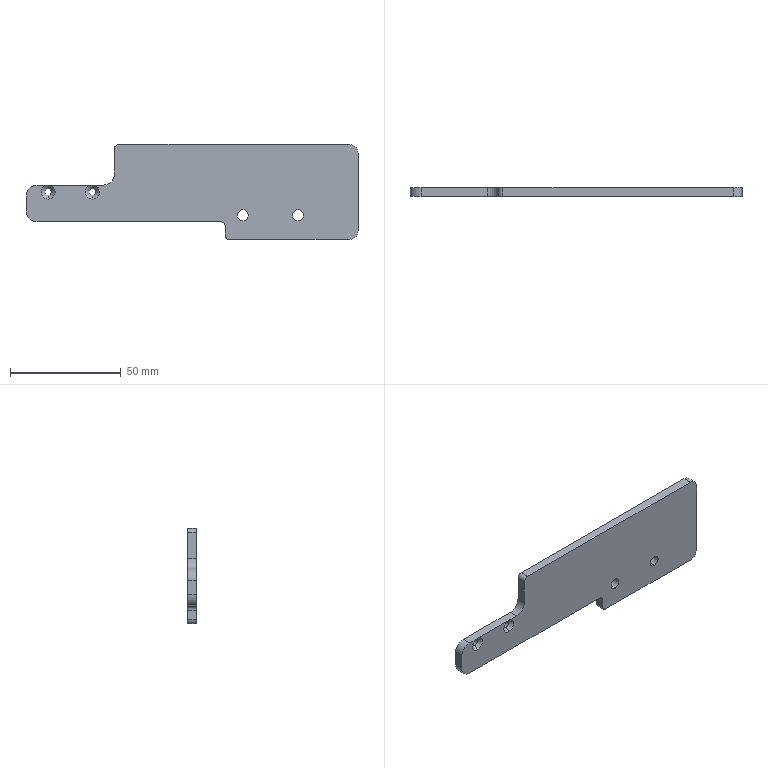Part | SolidWorks | features BaseBody 1 | 1 solid | 30 faces | box 150 x 4 x 43 mm | volume 19674 mm3 | cylinder 16 | plane 10 | cone 4 | commonest cylinder face diameters 3.1 x4 5 x4 4 x3 10 x3 8 x2
STEP:
#1=CARTESIAN_POINT('',(-78.,1.65,-1.55));
#2=VERTEX_POINT('',#1);
#3=CARTESIAN_POINT('',(-78.,1.65,1.55));
#4=VERTEX_POINT('',#3);
#5=CARTESIAN_POINT('',(-78.,1.65,0.));
#6=DIRECTION('',(0.,1.,0.));
#7=DIRECTION('',(0.,0.,1.));
#8=AXIS2_PLACEMENT_3D('',#5,#6,#7);
#9=CIRCLE('',#8,1.55);
#10=EDGE_CURVE('',#2,#4,#9,.T.);
#11=ORIENTED_EDGE('',*,*,#10,.F.);
#12=CARTESIAN_POINT('',(-78.,4.,-1.55));
#13=VERTEX_POINT('',#12);
#14=CARTESIAN_POINT('',(-78.,0.,-1.55));
#15=DIRECTION('',(0.,1.,0.));
#16=VECTOR('',#15,1000.);
#17=LINE('',#14,#16);
#18=EDGE_CURVE('',#2,#13,#17,.T.);
#19=ORIENTED_EDGE('',*,*,#18,.T.);
#20=CARTESIAN_POINT('',(-78.,4.,1.55));
#21=VERTEX_POINT('',#20);
#22=CARTESIAN_POINT('',(-78.,4.,0.));
#23=DIRECTION('',(0.,1.,0.));
#24=DIRECTION('',(0.,0.,1.));
#25=AXIS2_PLACEMENT_3D('',#22,#23,#24);
#26=CIRCLE('',#25,1.55);
#27=EDGE_CURVE('',#13,#21,#26,.T.);
#28=ORIENTED_EDGE('',*,*,#27,.T.);
#29=CARTESIAN_POINT('',(-78.,0.,1.55));
#30=DIRECTION('',(0.,1.,0.));
#31=VECTOR('',#30,1000.);
#32=LINE('',#29,#31);
#33=EDGE_CURVE('',#4,#21,#32,.T.);
#34=ORIENTED_EDGE('',*,*,#33,.F.);
#35=EDGE_LOOP('',(#11,#19,#28,#34));
#36=FACE_OUTER_BOUND('',#35,.T.);
#37=CARTESIAN_POINT('',(-78.,0.,0.));
#38=DIRECTION('',(0.,1.,0.));
#39=DIRECTION('',(0.,0.,1.));
#40=AXIS2_PLACEMENT_3D('',#37,#38,#39);
#41=CYLINDRICAL_SURFACE('',#40,1.55);
#42=ADVANCED_FACE('',(#36),#41,.F.);
#43=CARTESIAN_POINT('',(-98.,1.65,-1.55));
#44=VERTEX_POINT('',#43);
#45=CARTESIAN_POINT('',(-98.,1.65,1.55));
#46=VERTEX_POINT('',#45);
#47=CARTESIAN_POINT('',(-98.,1.65,0.));
#48=DIRECTION('',(0.,1.,0.));
#49=DIRECTION('',(0.,0.,1.));
#50=AXIS2_PLACEMENT_3D('',#47,#48,#49);
#51=CIRCLE('',#50,1.55);
#52=EDGE_CURVE('',#44,#46,#51,.T.);
#53=ORIENTED_EDGE('',*,*,#52,.F.);
#54=CARTESIAN_POINT('',(-98.,4.,-1.55));
#55=VERTEX_POINT('',#54);
#56=CARTESIAN_POINT('',(-98.,0.,-1.55));
#57=DIRECTION('',(0.,1.,0.));
#58=VECTOR('',#57,1000.);
#59=LINE('',#56,#58);
#60=EDGE_CURVE('',#44,#55,#59,.T.);
#61=ORIENTED_EDGE('',*,*,#60,.T.);
#62=CARTESIAN_POINT('',(-98.,4.,1.55));
#63=VERTEX_POINT('',#62);
#64=CARTESIAN_POINT('',(-98.,4.,0.));
#65=DIRECTION('',(0.,1.,0.));
#66=DIRECTION('',(0.,0.,1.));
#67=AXIS2_PLACEMENT_3D('',#64,#65,#66);
#68=CIRCLE('',#67,1.55);
#69=EDGE_CURVE('',#55,#63,#68,.T.);
#70=ORIENTED_EDGE('',*,*,#69,.T.);
#71=CARTESIAN_POINT('',(-98.,0.,1.55));
#72=DIRECTION('',(0.,1.,0.));
#73=VECTOR('',#72,1000.);
#74=LINE('',#71,#73);
#75=EDGE_CURVE('',#46,#63,#74,.T.);
#76=ORIENTED_EDGE('',*,*,#75,.F.);
#77=EDGE_LOOP('',(#53,#61,#70,#76));
#78=FACE_OUTER_BOUND('',#77,.T.);
#79=CARTESIAN_POINT('',(-98.,0.,0.));
#80=DIRECTION('',(0.,1.,0.));
#81=DIRECTION('',(0.,0.,1.));
#82=AXIS2_PLACEMENT_3D('',#79,#80,#81);
#83=CYLINDRICAL_SURFACE('',#82,1.55);
#84=ADVANCED_FACE('',(#78),#83,.F.);
#85=CARTESIAN_POINT('',(14.95,4.,-13.));
#86=VERTEX_POINT('',#85);
#87=CARTESIAN_POINT('',(14.95,4.,-8.));
#88=VERTEX_POINT('',#87);
#89=CARTESIAN_POINT('',(14.95,4.,-10.5));
#90=DIRECTION('',(0.,1.,0.));
#91=DIRECTION('',(0.,0.,-1.));
#92=AXIS2_PLACEMENT_3D('',#89,#90,#91);
#93=CIRCLE('',#92,2.5);
#94=EDGE_CURVE('',#86,#88,#93,.T.);
#95=ORIENTED_EDGE('',*,*,#94,.T.);
#96=CARTESIAN_POINT('',(14.95,0.,-8.));
#97=VERTEX_POINT('',#96);
#98=CARTESIAN_POINT('',(14.95,10.,-8.));
#99=DIRECTION('',(0.,-1.,0.));
#100=VECTOR('',#99,1000.);
#101=LINE('',#98,#100);
#102=EDGE_CURVE('',#88,#97,#101,.T.);
#103=ORIENTED_EDGE('',*,*,#102,.T.);
#104=CARTESIAN_POINT('',(14.95,0.,-13.));
#105=VERTEX_POINT('',#104);
#106=CARTESIAN_POINT('',(14.95,0.,-10.5));
#107=DIRECTION('',(0.,1.,0.));
#108=DIRECTION('',(0.,0.,-1.));
#109=AXIS2_PLACEMENT_3D('',#106,#107,#108);
#110=CIRCLE('',#109,2.5);
#111=EDGE_CURVE('',#105,#97,#110,.T.);
#112=ORIENTED_EDGE('',*,*,#111,.F.);
#113=CARTESIAN_POINT('',(14.95,10.,-13.));
#114=DIRECTION('',(0.,-1.,0.));
#115=VECTOR('',#114,1000.);
#116=LINE('',#113,#115);
#117=EDGE_CURVE('',#86,#105,#116,.T.);
#118=ORIENTED_EDGE('',*,*,#117,.F.);
#119=EDGE_LOOP('',(#95,#103,#112,#118));
#120=FACE_OUTER_BOUND('',#119,.T.);
#121=CARTESIAN_POINT('',(14.95,10.,-10.5));
#122=DIRECTION('',(0.,-1.,0.));
#123=DIRECTION('',(0.,0.,-1.));
#124=AXIS2_PLACEMENT_3D('',#121,#122,#123);
#125=CYLINDRICAL_SURFACE('',#124,2.5);
#126=ADVANCED_FACE('',(#120),#125,.F.);
#127=CARTESIAN_POINT('',(-10.05,4.,-13.));
#128=VERTEX_POINT('',#127);
#129=CARTESIAN_POINT('',(-10.05,4.,-8.));
#130=VERTEX_POINT('',#129);
#131=CARTESIAN_POINT('',(-10.05,4.,-10.5));
#132=DIRECTION('',(0.,1.,0.));
#133=DIRECTION('',(0.,0.,-1.));
#134=AXIS2_PLACEMENT_3D('',#131,#132,#133);
#135=CIRCLE('',#134,2.5);
#136=EDGE_CURVE('',#128,#130,#135,.T.);
#137=ORIENTED_EDGE('',*,*,#136,.T.);
#138=CARTESIAN_POINT('',(-10.05,0.,-8.));
#139=VERTEX_POINT('',#138);
#140=CARTESIAN_POINT('',(-10.05,10.,-8.));
#141=DIRECTION('',(0.,-1.,0.));
#142=VECTOR('',#141,1000.);
#143=LINE('',#140,#142);
#144=EDGE_CURVE('',#130,#139,#143,.T.);
#145=ORIENTED_EDGE('',*,*,#144,.T.);
#146=CARTESIAN_POINT('',(-10.05,0.,-13.));
#147=VERTEX_POINT('',#146);
#148=CARTESIAN_POINT('',(-10.05,0.,-10.5));
#149=DIRECTION('',(0.,1.,0.));
#150=DIRECTION('',(0.,0.,-1.));
#151=AXIS2_PLACEMENT_3D('',#148,#149,#150);
#152=CIRCLE('',#151,2.5);
#153=EDGE_CURVE('',#147,#139,#152,.T.);
#154=ORIENTED_EDGE('',*,*,#153,.F.);
#155=CARTESIAN_POINT('',(-10.05,10.,-13.));
#156=DIRECTION('',(0.,-1.,0.));
#157=VECTOR('',#156,1000.);
#158=LINE('',#155,#157);
#159=EDGE_CURVE('',#128,#147,#158,.T.);
#160=ORIENTED_EDGE('',*,*,#159,.F.);
#161=EDGE_LOOP('',(#137,#145,#154,#160));
#162=FACE_OUTER_BOUND('',#161,.T.);
#163=CARTESIAN_POINT('',(-10.05,10.,-10.5));
#164=DIRECTION('',(0.,-1.,0.));
#165=DIRECTION('',(0.,0.,-1.));
#166=AXIS2_PLACEMENT_3D('',#163,#164,#165);
#167=CYLINDRICAL_SURFACE('',#166,2.5);
#168=ADVANCED_FACE('',(#162),#167,.F.);
#169=ORIENTED_EDGE('',*,*,#10,.T.);
#170=CARTESIAN_POINT('',(-78.,0.07698,3.123));
#171=VERTEX_POINT('',#170);
#172=CARTESIAN_POINT('',(-78.,0.,3.2));
#173=DIRECTION('',(0.,-0.7071,0.7071));
#174=VECTOR('',#173,1000.);
#175=LINE('',#172,#174);
#176=EDGE_CURVE('',#4,#171,#175,.T.);
#177=ORIENTED_EDGE('',*,*,#176,.T.);
#178=CARTESIAN_POINT('',(-78.698,0.,3.123));
#179=VERTEX_POINT('',#178);
#180=CARTESIAN_POINT('',(-78.698,0.,3.123));
#181=CARTESIAN_POINT('',(-78.468,0.05012,3.123));
#182=CARTESIAN_POINT('',(-78.235,0.07698,3.123));
#183=CARTESIAN_POINT('',(-78.,0.07698,3.123));
#184=B_SPLINE_CURVE_WITH_KNOTS('',3,(#180,#181,#182,#183),.UNSPECIFIED.,.F.,.F.,(4,4),(-0.0007019,0.),.UNSPECIFIED.);
#185=EDGE_CURVE('',#179,#171,#184,.T.);
#186=ORIENTED_EDGE('',*,*,#185,.F.);
#187=CARTESIAN_POINT('',(-78.,0.,-3.2));
#188=VERTEX_POINT('',#187);
#189=CARTESIAN_POINT('',(-78.,0.,0.));
#190=DIRECTION('',(0.,1.,0.));
#191=DIRECTION('',(0.,0.,-1.));
#192=AXIS2_PLACEMENT_3D('',#189,#190,#191);
#193=CIRCLE('',#192,3.2);
#194=EDGE_CURVE('',#188,#179,#193,.T.);
#195=ORIENTED_EDGE('',*,*,#194,.F.);
#196=CARTESIAN_POINT('',(-78.,0.,-3.2));
#197=DIRECTION('',(0.,-0.7071,-0.7071));
#198=VECTOR('',#197,1000.);
#199=LINE('',#196,#198);
#200=EDGE_CURVE('',#2,#188,#199,.T.);
#201=ORIENTED_EDGE('',*,*,#200,.F.);
#202=EDGE_LOOP('',(#169,#177,#186,#195,#201));
#203=FACE_OUTER_BOUND('',#202,.T.);
#204=CARTESIAN_POINT('',(-78.,0.,0.));
#205=DIRECTION('',(0.,-1.,0.));
#206=DIRECTION('',(0.,0.,-1.));
#207=AXIS2_PLACEMENT_3D('',#204,#205,#206);
#208=CONICAL_SURFACE('',#207,3.2,0.7854);
#209=ADVANCED_FACE('',(#203),#208,.F.);
#210=ORIENTED_EDGE('',*,*,#52,.T.);
#211=CARTESIAN_POINT('',(-98.,0.07698,3.123));
#212=VERTEX_POINT('',#211);
#213=CARTESIAN_POINT('',(-98.,0.,3.2));
#214=DIRECTION('',(0.,-0.7071,0.7071));
#215=VECTOR('',#214,1000.);
#216=LINE('',#213,#215);
#217=EDGE_CURVE('',#46,#212,#216,.T.);
#218=ORIENTED_EDGE('',*,*,#217,.T.);
#219=CARTESIAN_POINT('',(-98.698,0.,3.123));
#220=VERTEX_POINT('',#219);
#221=CARTESIAN_POINT('',(-98.698,0.,3.123));
#222=CARTESIAN_POINT('',(-98.468,0.05012,3.123));
#223=CARTESIAN_POINT('',(-98.235,0.07698,3.123));
#224=CARTESIAN_POINT('',(-98.,0.07698,3.123));
#225=B_SPLINE_CURVE_WITH_KNOTS('',3,(#221,#222,#223,#224),.UNSPECIFIED.,.F.,.F.,(4,4),(-0.0007019,0.),.UNSPECIFIED.);
#226=EDGE_CURVE('',#220,#212,#225,.T.);
#227=ORIENTED_EDGE('',*,*,#226,.F.);
#228=CARTESIAN_POINT('',(-98.,0.,-3.2));
#229=VERTEX_POINT('',#228);
#230=CARTESIAN_POINT('',(-98.,0.,0.));
#231=DIRECTION('',(0.,1.,0.));
#232=DIRECTION('',(0.,0.,-1.));
#233=AXIS2_PLACEMENT_3D('',#230,#231,#232);
#234=CIRCLE('',#233,3.2);
#235=EDGE_CURVE('',#229,#220,#234,.T.);
#236=ORIENTED_EDGE('',*,*,#235,.F.);
#237=CARTESIAN_POINT('',(-98.,0.,-3.2));
#238=DIRECTION('',(0.,-0.7071,-0.7071));
#239=VECTOR('',#238,1000.);
#240=LINE('',#237,#239);
#241=EDGE_CURVE('',#44,#229,#240,.T.);
#242=ORIENTED_EDGE('',*,*,#241,.F.);
#243=EDGE_LOOP('',(#210,#218,#227,#236,#242));
#244=FACE_OUTER_BOUND('',#243,.T.);
#245=CARTESIAN_POINT('',(-98.,0.,0.));
#246=DIRECTION('',(0.,-1.,0.));
#247=DIRECTION('',(0.,0.,-1.));
#248=AXIS2_PLACEMENT_3D('',#245,#246,#247);
#249=CONICAL_SURFACE('',#248,3.2,0.7854);
#250=ADVANCED_FACE('',(#244),#249,.F.);
#251=CARTESIAN_POINT('',(-103.,4.,3.123));
#252=VERTEX_POINT('',#251);
#253=CARTESIAN_POINT('',(-108.,4.,-1.877));
#254=VERTEX_POINT('',#253);
#255=CARTESIAN_POINT('',(-103.,4.,-1.877));
#256=DIRECTION('',(0.,-1.,0.));
#257=DIRECTION('',(0.,0.,-1.));
#258=AXIS2_PLACEMENT_3D('',#255,#256,#257);
#259=CIRCLE('',#258,5.);
#260=EDGE_CURVE('',#252,#254,#259,.T.);
#261=ORIENTED_EDGE('',*,*,#260,.F.);
#262=CARTESIAN_POINT('',(-73.,4.,3.123));
#263=VERTEX_POINT('',#262);
#264=CARTESIAN_POINT('',(0.,4.,3.123));
#265=DIRECTION('',(-1.,0.,0.));
#266=VECTOR('',#265,1000.);
#267=LINE('',#264,#266);
#268=EDGE_CURVE('',#263,#252,#267,.T.);
#269=ORIENTED_EDGE('',*,*,#268,.F.);
#270=CARTESIAN_POINT('',(-68.,4.,8.123));
#271=VERTEX_POINT('',#270);
#272=CARTESIAN_POINT('',(-73.,4.,8.123));
#273=DIRECTION('',(0.,1.,0.));
#274=DIRECTION('',(0.,0.,-1.));
#275=AXIS2_PLACEMENT_3D('',#272,#273,#274);
#276=CIRCLE('',#275,5.);
#277=EDGE_CURVE('',#271,#263,#276,.T.);
#278=ORIENTED_EDGE('',*,*,#277,.F.);
#279=CARTESIAN_POINT('',(-68.,4.,19.5));
#280=VERTEX_POINT('',#279);
#281=CARTESIAN_POINT('',(-68.,4.,0.));
#282=DIRECTION('',(0.,0.,-1.));
#283=VECTOR('',#282,1000.);
#284=LINE('',#281,#283);
#285=EDGE_CURVE('',#280,#271,#284,.T.);
#286=ORIENTED_EDGE('',*,*,#285,.F.);
#287=CARTESIAN_POINT('',(-66.,4.,21.5));
#288=VERTEX_POINT('',#287);
#289=CARTESIAN_POINT('',(-66.,4.,19.5));
#290=DIRECTION('',(0.,-1.,0.));
#291=DIRECTION('',(0.,0.,-1.));
#292=AXIS2_PLACEMENT_3D('',#289,#290,#291);
#293=CIRCLE('',#292,2.);
#294=EDGE_CURVE('',#288,#280,#293,.T.);
#295=ORIENTED_EDGE('',*,*,#294,.F.);
#296=CARTESIAN_POINT('',(38.,4.,21.5));
#297=VERTEX_POINT('',#296);
#298=CARTESIAN_POINT('',(0.,4.,21.5));
#299=DIRECTION('',(-1.,0.,0.));
#300=VECTOR('',#299,1000.);
#301=LINE('',#298,#300);
#302=EDGE_CURVE('',#297,#288,#301,.T.);
#303=ORIENTED_EDGE('',*,*,#302,.F.);
#304=CARTESIAN_POINT('',(42.,4.,17.5));
#305=VERTEX_POINT('',#304);
#306=CARTESIAN_POINT('',(38.,4.,17.5));
#307=DIRECTION('',(0.,-1.,0.));
#308=DIRECTION('',(0.,0.,1.));
#309=AXIS2_PLACEMENT_3D('',#306,#307,#308);
#310=CIRCLE('',#309,4.);
#311=EDGE_CURVE('',#305,#297,#310,.T.);
#312=ORIENTED_EDGE('',*,*,#311,.F.);
#313=CARTESIAN_POINT('',(42.,4.,-17.5));
#314=VERTEX_POINT('',#313);
#315=CARTESIAN_POINT('',(42.,4.,0.));
#316=DIRECTION('',(0.,0.,1.));
#317=VECTOR('',#316,1000.);
#318=LINE('',#315,#317);
#319=EDGE_CURVE('',#314,#305,#318,.T.);
#320=ORIENTED_EDGE('',*,*,#319,.F.);
#321=CARTESIAN_POINT('',(38.,4.,-21.5));
#322=VERTEX_POINT('',#321);
#323=CARTESIAN_POINT('',(38.,4.,-17.5));
#324=DIRECTION('',(0.,-1.,0.));
#325=DIRECTION('',(0.,0.,1.));
#326=AXIS2_PLACEMENT_3D('',#323,#324,#325);
#327=CIRCLE('',#326,4.);
#328=EDGE_CURVE('',#322,#314,#327,.T.);
#329=ORIENTED_EDGE('',*,*,#328,.F.);
#330=CARTESIAN_POINT('',(-16.,4.,-21.5));
#331=VERTEX_POINT('',#330);
#332=CARTESIAN_POINT('',(0.,4.,-21.5));
#333=DIRECTION('',(1.,0.,0.));
#334=VECTOR('',#333,1000.);
#335=LINE('',#332,#334);
#336=EDGE_CURVE('',#331,#322,#335,.T.);
#337=ORIENTED_EDGE('',*,*,#336,.F.);
#338=CARTESIAN_POINT('',(-18.,4.,-19.5));
#339=VERTEX_POINT('',#338);
#340=CARTESIAN_POINT('',(-16.,4.,-19.5));
#341=DIRECTION('',(0.,-1.,0.));
#342=DIRECTION('',(0.,0.,1.));
#343=AXIS2_PLACEMENT_3D('',#340,#341,#342);
#344=CIRCLE('',#343,2.);
#345=EDGE_CURVE('',#339,#331,#344,.T.);
#346=ORIENTED_EDGE('',*,*,#345,.F.);
#347=CARTESIAN_POINT('',(-18.,4.,-15.5));
#348=VERTEX_POINT('',#347);
#349=CARTESIAN_POINT('',(-18.,4.,0.));
#350=DIRECTION('',(0.,0.,-1.));
#351=VECTOR('',#350,1000.);
#352=LINE('',#349,#351);
#353=EDGE_CURVE('',#348,#339,#352,.T.);
#354=ORIENTED_EDGE('',*,*,#353,.F.);
#355=CARTESIAN_POINT('',(-20.,4.,-13.5));
#356=VERTEX_POINT('',#355);
#357=CARTESIAN_POINT('',(-20.,4.,-15.5));
#358=DIRECTION('',(0.,1.,0.));
#359=DIRECTION('',(0.,0.,-1.));
#360=AXIS2_PLACEMENT_3D('',#357,#358,#359);
#361=CIRCLE('',#360,2.);
#362=EDGE_CURVE('',#356,#348,#361,.T.);
#363=ORIENTED_EDGE('',*,*,#362,.F.);
#364=CARTESIAN_POINT('',(-103.,4.,-13.5));
#365=VERTEX_POINT('',#364);
#366=CARTESIAN_POINT('',(0.,4.,-13.5));
#367=DIRECTION('',(1.,0.,0.));
#368=VECTOR('',#367,1000.);
#369=LINE('',#366,#368);
#370=EDGE_CURVE('',#365,#356,#369,.T.);
#371=ORIENTED_EDGE('',*,*,#370,.F.);
#372=CARTESIAN_POINT('',(-108.,4.,-8.5));
#373=VERTEX_POINT('',#372);
#374=CARTESIAN_POINT('',(-103.,4.,-8.5));
#375=DIRECTION('',(0.,-1.,0.));
#376=DIRECTION('',(0.,0.,-1.));
#377=AXIS2_PLACEMENT_3D('',#374,#375,#376);
#378=CIRCLE('',#377,5.);
#379=EDGE_CURVE('',#373,#365,#378,.T.);
#380=ORIENTED_EDGE('',*,*,#379,.F.);
#381=CARTESIAN_POINT('',(-108.,4.,0.));
#382=DIRECTION('',(0.,0.,-1.));
#383=VECTOR('',#382,1000.);
#384=LINE('',#381,#383);
#385=EDGE_CURVE('',#254,#373,#384,.T.);
#386=ORIENTED_EDGE('',*,*,#385,.F.);
#387=EDGE_LOOP('',(#261,#269,#278,#286,#295,#303,#312,#320,#329,#337,#346,#354,#363,#371,#380,#386));
#388=FACE_OUTER_BOUND('',#387,.T.);
#389=CARTESIAN_POINT('',(-78.,4.,0.));
#390=DIRECTION('',(0.,1.,0.));
#391=DIRECTION('',(0.,0.,1.));
#392=AXIS2_PLACEMENT_3D('',#389,#390,#391);
#393=CIRCLE('',#392,1.55);
#394=EDGE_CURVE('',#21,#13,#393,.T.);
#395=ORIENTED_EDGE('',*,*,#394,.F.);
#396=ORIENTED_EDGE('',*,*,#27,.F.);
#397=EDGE_LOOP('',(#395,#396));
#398=FACE_BOUND('',#397,.T.);
#399=CARTESIAN_POINT('',(-98.,4.,0.));
#400=DIRECTION('',(0.,1.,0.));
#401=DIRECTION('',(0.,0.,1.));
#402=AXIS2_PLACEMENT_3D('',#399,#400,#401);
#403=CIRCLE('',#402,1.55);
#404=EDGE_CURVE('',#63,#55,#403,.T.);
#405=ORIENTED_EDGE('',*,*,#404,.F.);
#406=ORIENTED_EDGE('',*,*,#69,.F.);
#407=EDGE_LOOP('',(#405,#406));
#408=FACE_BOUND('',#407,.T.);
#409=ORIENTED_EDGE('',*,*,#94,.F.);
#410=CARTESIAN_POINT('',(14.95,4.,-10.5));
#411=DIRECTION('',(0.,1.,0.));
#412=DIRECTION('',(0.,0.,-1.));
#413=AXIS2_PLACEMENT_3D('',#410,#411,#412);
#414=CIRCLE('',#413,2.5);
#415=EDGE_CURVE('',#88,#86,#414,.T.);
#416=ORIENTED_EDGE('',*,*,#415,.F.);
#417=EDGE_LOOP('',(#409,#416));
#418=FACE_BOUND('',#417,.T.);
#419=ORIENTED_EDGE('',*,*,#136,.F.);
#420=CARTESIAN_POINT('',(-10.05,4.,-10.5));
#421=DIRECTION('',(0.,1.,0.));
#422=DIRECTION('',(0.,0.,-1.));
#423=AXIS2_PLACEMENT_3D('',#420,#421,#422);
#424=CIRCLE('',#423,2.5);
#425=EDGE_CURVE('',#130,#128,#424,.T.);
#426=ORIENTED_EDGE('',*,*,#425,.F.);
#427=EDGE_LOOP('',(#419,#426));
#428=FACE_BOUND('',#427,.T.);
#429=CARTESIAN_POINT('',(0.,4.,0.));
#430=DIRECTION('',(0.,-1.,0.));
#431=DIRECTION('',(0.,0.,-1.));
#432=AXIS2_PLACEMENT_3D('',#429,#430,#431);
#433=PLANE('',#432);
#434=ADVANCED_FACE('',(#388,#398,#408,#418,#428),#433,.F.);
#435=ORIENTED_EDGE('',*,*,#385,.T.);
#436=CARTESIAN_POINT('',(-108.,0.,-8.5));
#437=VERTEX_POINT('',#436);
#438=CARTESIAN_POINT('',(-108.,0.,-8.5));
#439=DIRECTION('',(0.,-1.,0.));
#440=VECTOR('',#439,1000.);
#441=LINE('',#438,#440);
#442=EDGE_CURVE('',#373,#437,#441,.T.);
#443=ORIENTED_EDGE('',*,*,#442,.T.);
#444=CARTESIAN_POINT('',(-108.,0.,-1.877));
#445=VERTEX_POINT('',#444);
#446=CARTESIAN_POINT('',(-108.,0.,-21.5));
#447=DIRECTION('',(0.,0.,1.));
#448=VECTOR('',#447,1000.);
#449=LINE('',#446,#448);
#450=EDGE_CURVE('',#437,#445,#449,.T.);
#451=ORIENTED_EDGE('',*,*,#450,.T.);
#452=CARTESIAN_POINT('',(-108.,0.,-1.877));
#453=DIRECTION('',(0.,1.,0.));
#454=VECTOR('',#453,1000.);
#455=LINE('',#452,#454);
#456=EDGE_CURVE('',#445,#254,#455,.T.);
#457=ORIENTED_EDGE('',*,*,#456,.T.);
#458=EDGE_LOOP('',(#435,#443,#451,#457));
#459=FACE_OUTER_BOUND('',#458,.T.);
#460=CARTESIAN_POINT('',(-108.,0.,-21.5));
#461=DIRECTION('',(-1.,0.,0.));
#462=DIRECTION('',(0.,0.,1.));
#463=AXIS2_PLACEMENT_3D('',#460,#461,#462);
#464=PLANE('',#463);
#465=ADVANCED_FACE('',(#459),#464,.T.);
#466=ORIENTED_EDGE('',*,*,#260,.T.);
#467=ORIENTED_EDGE('',*,*,#456,.F.);
#468=CARTESIAN_POINT('',(-103.,0.,3.123));
#469=VERTEX_POINT('',#468);
#470=CARTESIAN_POINT('',(-103.,0.,-1.877));
#471=DIRECTION('',(0.,1.,0.));
#472=DIRECTION('',(0.,0.,-1.));
#473=AXIS2_PLACEMENT_3D('',#470,#471,#472);
#474=CIRCLE('',#473,5.);
#475=EDGE_CURVE('',#445,#469,#474,.T.);
#476=ORIENTED_EDGE('',*,*,#475,.T.);
#477=CARTESIAN_POINT('',(-103.,0.,3.123));
#478=DIRECTION('',(0.,1.,0.));
#479=VECTOR('',#478,1000.);
#480=LINE('',#477,#479);
#481=EDGE_CURVE('',#469,#252,#480,.T.);
#482=ORIENTED_EDGE('',*,*,#481,.T.);
#483=EDGE_LOOP('',(#466,#467,#476,#482));
#484=FACE_OUTER_BOUND('',#483,.T.);
#485=CARTESIAN_POINT('',(-103.,0.,-1.877));
#486=DIRECTION('',(0.,-1.,0.));
#487=DIRECTION('',(0.,0.,-1.));
#488=AXIS2_PLACEMENT_3D('',#485,#486,#487);
#489=CYLINDRICAL_SURFACE('',#488,5.);
#490=ADVANCED_FACE('',(#484),#489,.T.);
#491=ORIENTED_EDGE('',*,*,#481,.F.);
#492=CARTESIAN_POINT('',(-68.,0.,3.123));
#493=DIRECTION('',(-1.,0.,0.));
#494=VECTOR('',#493,1000.);
#495=LINE('',#492,#494);
#496=EDGE_CURVE('',#220,#469,#495,.T.);
#497=ORIENTED_EDGE('',*,*,#496,.F.);
#498=ORIENTED_EDGE('',*,*,#226,.T.);
#499=CARTESIAN_POINT('',(-97.302,0.,3.123));
#500=VERTEX_POINT('',#499);
#501=CARTESIAN_POINT('',(-98.,0.07698,3.123));
#502=CARTESIAN_POINT('',(-97.765,0.07698,3.123));
#503=CARTESIAN_POINT('',(-97.532,0.05012,3.123));
#504=CARTESIAN_POINT('',(-97.302,0.,3.123));
#505=B_SPLINE_CURVE_WITH_KNOTS('',3,(#501,#502,#503,#504),.UNSPECIFIED.,.F.,.F.,(4,4),(0.,0.0007019),.UNSPECIFIED.);
#506=EDGE_CURVE('',#212,#500,#505,.T.);
#507=ORIENTED_EDGE('',*,*,#506,.T.);
#508=CARTESIAN_POINT('',(-68.,0.,3.123));
#509=DIRECTION('',(-1.,0.,0.));
#510=VECTOR('',#509,1000.);
#511=LINE('',#508,#510);
#512=EDGE_CURVE('',#179,#500,#511,.T.);
#513=ORIENTED_EDGE('',*,*,#512,.F.);
#514=ORIENTED_EDGE('',*,*,#185,.T.);
#515=CARTESIAN_POINT('',(-77.302,0.,3.123));
#516=VERTEX_POINT('',#515);
#517=CARTESIAN_POINT('',(-78.,0.07698,3.123));
#518=CARTESIAN_POINT('',(-77.765,0.07698,3.123));
#519=CARTESIAN_POINT('',(-77.532,0.05012,3.123));
#520=CARTESIAN_POINT('',(-77.302,0.,3.123));
#521=B_SPLINE_CURVE_WITH_KNOTS('',3,(#517,#518,#519,#520),.UNSPECIFIED.,.F.,.F.,(4,4),(0.,0.0007019),.UNSPECIFIED.);
#522=EDGE_CURVE('',#171,#516,#521,.T.);
#523=ORIENTED_EDGE('',*,*,#522,.T.);
#524=CARTESIAN_POINT('',(-73.,0.,3.123));
#525=VERTEX_POINT('',#524);
#526=CARTESIAN_POINT('',(-68.,0.,3.123));
#527=DIRECTION('',(-1.,0.,0.));
#528=VECTOR('',#527,1000.);
#529=LINE('',#526,#528);
#530=EDGE_CURVE('',#525,#516,#529,.T.);
#531=ORIENTED_EDGE('',*,*,#530,.F.);
#532=CARTESIAN_POINT('',(-73.,-6.,3.123));
#533=DIRECTION('',(0.,-1.,0.));
#534=VECTOR('',#533,1000.);
#535=LINE('',#532,#534);
#536=EDGE_CURVE('',#263,#525,#535,.T.);
#537=ORIENTED_EDGE('',*,*,#536,.F.);
#538=ORIENTED_EDGE('',*,*,#268,.T.);
#539=EDGE_LOOP('',(#491,#497,#498,#507,#513,#514,#523,#531,#537,#538));
#540=FACE_OUTER_BOUND('',#539,.T.);
#541=CARTESIAN_POINT('',(-68.,-6.,3.123));
#542=DIRECTION('',(0.,0.,-1.));
#543=DIRECTION('',(-1.,0.,0.));
#544=AXIS2_PLACEMENT_3D('',#541,#542,#543);
#545=PLANE('',#544);
#546=ADVANCED_FACE('',(#540),#545,.F.);
#547=CARTESIAN_POINT('',(-68.,0.,8.123));
#548=VERTEX_POINT('',#547);
#549=CARTESIAN_POINT('',(-68.,-6.,8.123));
#550=DIRECTION('',(0.,-1.,0.));
#551=VECTOR('',#550,1000.);
#552=LINE('',#549,#551);
#553=EDGE_CURVE('',#271,#548,#552,.T.);
#554=ORIENTED_EDGE('',*,*,#553,.F.);
#555=ORIENTED_EDGE('',*,*,#277,.T.);
#556=ORIENTED_EDGE('',*,*,#536,.T.);
#557=CARTESIAN_POINT('',(-73.,0.,8.123));
#558=DIRECTION('',(0.,1.,0.));
#559=DIRECTION('',(0.,0.,-1.));
#560=AXIS2_PLACEMENT_3D('',#557,#558,#559);
#561=CIRCLE('',#560,5.);
#562=EDGE_CURVE('',#548,#525,#561,.T.);
#563=ORIENTED_EDGE('',*,*,#562,.F.);
#564=EDGE_LOOP('',(#554,#555,#556,#563));
#565=FACE_OUTER_BOUND('',#564,.T.);
#566=CARTESIAN_POINT('',(-73.,-6.,8.123));
#567=DIRECTION('',(0.,-1.,0.));
#568=DIRECTION('',(0.,0.,-1.));
#569=AXIS2_PLACEMENT_3D('',#566,#567,#568);
#570=CYLINDRICAL_SURFACE('',#569,5.);
#571=ADVANCED_FACE('',(#565),#570,.F.);
#572=ORIENTED_EDGE('',*,*,#553,.T.);
#573=CARTESIAN_POINT('',(-68.,0.,19.5));
#574=VERTEX_POINT('',#573);
#575=CARTESIAN_POINT('',(-68.,0.,28.));
#576=DIRECTION('',(0.,0.,-1.));
#577=VECTOR('',#576,1000.);
#578=LINE('',#575,#577);
#579=EDGE_CURVE('',#574,#548,#578,.T.);
#580=ORIENTED_EDGE('',*,*,#579,.F.);
#581=CARTESIAN_POINT('',(-68.,-6.,19.5));
#582=DIRECTION('',(0.,-1.,0.));
#583=VECTOR('',#582,1000.);
#584=LINE('',#581,#583);
#585=EDGE_CURVE('',#280,#574,#584,.T.);
#586=ORIENTED_EDGE('',*,*,#585,.F.);
#587=ORIENTED_EDGE('',*,*,#285,.T.);
#588=EDGE_LOOP('',(#572,#580,#586,#587));
#589=FACE_OUTER_BOUND('',#588,.T.);
#590=CARTESIAN_POINT('',(-68.,-6.,28.));
#591=DIRECTION('',(1.,0.,0.));
#592=DIRECTION('',(0.,0.,-1.));
#593=AXIS2_PLACEMENT_3D('',#590,#591,#592);
#594=PLANE('',#593);
#595=ADVANCED_FACE('',(#589),#594,.F.);
#596=CARTESIAN_POINT('',(-66.,0.,21.5));
#597=VERTEX_POINT('',#596);
#598=CARTESIAN_POINT('',(-66.,0.,19.5));
#599=DIRECTION('',(0.,1.,0.));
#600=DIRECTION('',(0.,0.,-1.));
#601=AXIS2_PLACEMENT_3D('',#598,#599,#600);
#602=CIRCLE('',#601,2.);
#603=EDGE_CURVE('',#574,#597,#602,.T.);
#604=ORIENTED_EDGE('',*,*,#603,.T.);
#605=CARTESIAN_POINT('',(-66.,4.,21.5));
#606=DIRECTION('',(0.,1.,0.));
#607=VECTOR('',#606,1000.);
#608=LINE('',#605,#607);
#609=EDGE_CURVE('',#597,#288,#608,.T.);
#610=ORIENTED_EDGE('',*,*,#609,.T.);
#611=ORIENTED_EDGE('',*,*,#294,.T.);
#612=ORIENTED_EDGE('',*,*,#585,.T.);
#613=EDGE_LOOP('',(#604,#610,#611,#612));
#614=FACE_OUTER_BOUND('',#613,.T.);
#615=CARTESIAN_POINT('',(-66.,4.,19.5));
#616=DIRECTION('',(0.,-1.,0.));
#617=DIRECTION('',(0.,0.,-1.));
#618=AXIS2_PLACEMENT_3D('',#615,#616,#617);
#619=CYLINDRICAL_SURFACE('',#618,2.);
#620=ADVANCED_FACE('',(#614),#619,.T.);
#621=CARTESIAN_POINT('',(38.,0.,21.5));
#622=VERTEX_POINT('',#621);
#623=CARTESIAN_POINT('',(38.,4.,21.5));
#624=DIRECTION('',(0.,-1.,0.));
#625=VECTOR('',#624,1000.);
#626=LINE('',#623,#625);
#627=EDGE_CURVE('',#297,#622,#626,.T.);
#628=ORIENTED_EDGE('',*,*,#627,.F.);
#629=ORIENTED_EDGE('',*,*,#302,.T.);
#630=ORIENTED_EDGE('',*,*,#609,.F.);
#631=CARTESIAN_POINT('',(-90.,0.,21.5));
#632=DIRECTION('',(-1.,0.,0.));
#633=VECTOR('',#632,1000.);
#634=LINE('',#631,#633);
#635=EDGE_CURVE('',#622,#597,#634,.T.);
#636=ORIENTED_EDGE('',*,*,#635,.F.);
#637=EDGE_LOOP('',(#628,#629,#630,#636));
#638=FACE_OUTER_BOUND('',#637,.T.);
#639=CARTESIAN_POINT('',(-90.,4.,21.5));
#640=DIRECTION('',(0.,0.,-1.));
#641=DIRECTION('',(-1.,0.,0.));
#642=AXIS2_PLACEMENT_3D('',#639,#640,#641);
#643=PLANE('',#642);
#644=ADVANCED_FACE('',(#638),#643,.F.);
#645=ORIENTED_EDGE('',*,*,#311,.T.);
#646=ORIENTED_EDGE('',*,*,#627,.T.);
#647=CARTESIAN_POINT('',(42.,0.,17.5));
#648=VERTEX_POINT('',#647);
#649=CARTESIAN_POINT('',(38.,0.,17.5));
#650=DIRECTION('',(0.,1.,0.));
#651=DIRECTION('',(0.,0.,1.));
#652=AXIS2_PLACEMENT_3D('',#649,#650,#651);
#653=CIRCLE('',#652,4.);
#654=EDGE_CURVE('',#622,#648,#653,.T.);
#655=ORIENTED_EDGE('',*,*,#654,.T.);
#656=CARTESIAN_POINT('',(42.,4.,17.5));
#657=DIRECTION('',(0.,1.,0.));
#658=VECTOR('',#657,1000.);
#659=LINE('',#656,#658);
#660=EDGE_CURVE('',#648,#305,#659,.T.);
#661=ORIENTED_EDGE('',*,*,#660,.T.);
#662=EDGE_LOOP('',(#645,#646,#655,#661));
#663=FACE_OUTER_BOUND('',#662,.T.);
#664=CARTESIAN_POINT('',(38.,4.,17.5));
#665=DIRECTION('',(0.,1.,0.));
#666=DIRECTION('',(0.,0.,1.));
#667=AXIS2_PLACEMENT_3D('',#664,#665,#666);
#668=CYLINDRICAL_SURFACE('',#667,4.);
#669=ADVANCED_FACE('',(#663),#668,.T.);
#670=ORIENTED_EDGE('',*,*,#660,.F.);
#671=CARTESIAN_POINT('',(42.,0.,-17.5));
#672=VERTEX_POINT('',#671);
#673=CARTESIAN_POINT('',(42.,0.,-21.5));
#674=DIRECTION('',(0.,0.,1.));
#675=VECTOR('',#674,1000.);
#676=LINE('',#673,#675);
#677=EDGE_CURVE('',#672,#648,#676,.T.);
#678=ORIENTED_EDGE('',*,*,#677,.F.);
#679=CARTESIAN_POINT('',(42.,0.,-17.5));
#680=DIRECTION('',(0.,-1.,0.));
#681=VECTOR('',#680,1000.);
#682=LINE('',#679,#681);
#683=EDGE_CURVE('',#314,#672,#682,.T.);
#684=ORIENTED_EDGE('',*,*,#683,.F.);
#685=ORIENTED_EDGE('',*,*,#319,.T.);
#686=EDGE_LOOP('',(#670,#678,#684,#685));
#687=FACE_OUTER_BOUND('',#686,.T.);
#688=CARTESIAN_POINT('',(42.,0.,-21.5));
#689=DIRECTION('',(-1.,0.,0.));
#690=DIRECTION('',(0.,0.,1.));
#691=AXIS2_PLACEMENT_3D('',#688,#689,#690);
#692=PLANE('',#691);
#693=ADVANCED_FACE('',(#687),#692,.F.);
#694=ORIENTED_EDGE('',*,*,#328,.T.);
#695=ORIENTED_EDGE('',*,*,#683,.T.);
#696=CARTESIAN_POINT('',(38.,0.,-21.5));
#697=VERTEX_POINT('',#696);
#698=CARTESIAN_POINT('',(38.,0.,-17.5));
#699=DIRECTION('',(0.,1.,0.));
#700=DIRECTION('',(0.,0.,1.));
#701=AXIS2_PLACEMENT_3D('',#698,#699,#700);
#702=CIRCLE('',#701,4.);
#703=EDGE_CURVE('',#672,#697,#702,.T.);
#704=ORIENTED_EDGE('',*,*,#703,.T.);
#705=CARTESIAN_POINT('',(38.,0.,-21.5));
#706=DIRECTION('',(0.,1.,0.));
#707=VECTOR('',#706,1000.);
#708=LINE('',#705,#707);
#709=EDGE_CURVE('',#697,#322,#708,.T.);
#710=ORIENTED_EDGE('',*,*,#709,.T.);
#711=EDGE_LOOP('',(#694,#695,#704,#710));
#712=FACE_OUTER_BOUND('',#711,.T.);
#713=CARTESIAN_POINT('',(38.,0.,-17.5));
#714=DIRECTION('',(0.,1.,0.));
#715=DIRECTION('',(0.,0.,1.));
#716=AXIS2_PLACEMENT_3D('',#713,#714,#715);
#717=CYLINDRICAL_SURFACE('',#716,4.);
#718=ADVANCED_FACE('',(#712),#717,.T.);
#719=CARTESIAN_POINT('',(-16.,0.,-21.5));
#720=VERTEX_POINT('',#719);
#721=CARTESIAN_POINT('',(-16.,4.,-21.5));
#722=DIRECTION('',(0.,-1.,0.));
#723=VECTOR('',#722,1000.);
#724=LINE('',#721,#723);
#725=EDGE_CURVE('',#331,#720,#724,.T.);
#726=ORIENTED_EDGE('',*,*,#725,.F.);
#727=ORIENTED_EDGE('',*,*,#336,.T.);
#728=ORIENTED_EDGE('',*,*,#709,.F.);
#729=CARTESIAN_POINT('',(-90.,0.,-21.5));
#730=DIRECTION('',(1.,0.,0.));
#731=VECTOR('',#730,1000.);
#732=LINE('',#729,#731);
#733=EDGE_CURVE('',#720,#697,#732,.T.);
#734=ORIENTED_EDGE('',*,*,#733,.F.);
#735=EDGE_LOOP('',(#726,#727,#728,#734));
#736=FACE_OUTER_BOUND('',#735,.T.);
#737=CARTESIAN_POINT('',(-90.,4.,-21.5));
#738=DIRECTION('',(0.,0.,1.));
#739=DIRECTION('',(1.,0.,0.));
#740=AXIS2_PLACEMENT_3D('',#737,#738,#739);
#741=PLANE('',#740);
#742=ADVANCED_FACE('',(#736),#741,.F.);
#743=ORIENTED_EDGE('',*,*,#345,.T.);
#744=ORIENTED_EDGE('',*,*,#725,.T.);
#745=CARTESIAN_POINT('',(-18.,0.,-19.5));
#746=VERTEX_POINT('',#745);
#747=CARTESIAN_POINT('',(-16.,0.,-19.5));
#748=DIRECTION('',(0.,1.,0.));
#749=DIRECTION('',(0.,0.,1.));
#750=AXIS2_PLACEMENT_3D('',#747,#748,#749);
#751=CIRCLE('',#750,2.);
#752=EDGE_CURVE('',#720,#746,#751,.T.);
#753=ORIENTED_EDGE('',*,*,#752,.T.);
#754=CARTESIAN_POINT('',(-18.,4.,-19.5));
#755=DIRECTION('',(0.,1.,0.));
#756=VECTOR('',#755,1000.);
#757=LINE('',#754,#756);
#758=EDGE_CURVE('',#746,#339,#757,.T.);
#759=ORIENTED_EDGE('',*,*,#758,.T.);
#760=EDGE_LOOP('',(#743,#744,#753,#759));
#761=FACE_OUTER_BOUND('',#760,.T.);
#762=CARTESIAN_POINT('',(-16.,4.,-19.5));
#763=DIRECTION('',(0.,1.,0.));
#764=DIRECTION('',(0.,0.,1.));
#765=AXIS2_PLACEMENT_3D('',#762,#763,#764);
#766=CYLINDRICAL_SURFACE('',#765,2.);
#767=ADVANCED_FACE('',(#761),#766,.T.);
#768=ORIENTED_EDGE('',*,*,#758,.F.);
#769=CARTESIAN_POINT('',(-18.,0.,-15.5));
#770=VERTEX_POINT('',#769);
#771=CARTESIAN_POINT('',(-18.,0.,-13.5));
#772=DIRECTION('',(0.,0.,-1.));
#773=VECTOR('',#772,1000.);
#774=LINE('',#771,#773);
#775=EDGE_CURVE('',#770,#746,#774,.T.);
#776=ORIENTED_EDGE('',*,*,#775,.F.);
#777=CARTESIAN_POINT('',(-18.,-6.,-15.5));
#778=DIRECTION('',(0.,-1.,0.));
#779=VECTOR('',#778,1000.);
#780=LINE('',#777,#779);
#781=EDGE_CURVE('',#348,#770,#780,.T.);
#782=ORIENTED_EDGE('',*,*,#781,.F.);
#783=ORIENTED_EDGE('',*,*,#353,.T.);
#784=EDGE_LOOP('',(#768,#776,#782,#783));
#785=FACE_OUTER_BOUND('',#784,.T.);
#786=CARTESIAN_POINT('',(-18.,-6.,-13.5));
#787=DIRECTION('',(1.,0.,0.));
#788=DIRECTION('',(0.,0.,-1.));
#789=AXIS2_PLACEMENT_3D('',#786,#787,#788);
#790=PLANE('',#789);
#791=ADVANCED_FACE('',(#785),#790,.F.);
#792=CARTESIAN_POINT('',(-20.,0.,-13.5));
#793=VERTEX_POINT('',#792);
#794=CARTESIAN_POINT('',(-20.,-6.,-13.5));
#795=DIRECTION('',(0.,-1.,0.));
#796=VECTOR('',#795,1000.);
#797=LINE('',#794,#796);
#798=EDGE_CURVE('',#356,#793,#797,.T.);
#799=ORIENTED_EDGE('',*,*,#798,.F.);
#800=ORIENTED_EDGE('',*,*,#362,.T.);
#801=ORIENTED_EDGE('',*,*,#781,.T.);
#802=CARTESIAN_POINT('',(-20.,0.,-15.5));
#803=DIRECTION('',(0.,1.,0.));
#804=DIRECTION('',(0.,0.,-1.));
#805=AXIS2_PLACEMENT_3D('',#802,#803,#804);
#806=CIRCLE('',#805,2.);
#807=EDGE_CURVE('',#793,#770,#806,.T.);
#808=ORIENTED_EDGE('',*,*,#807,.F.);
#809=EDGE_LOOP('',(#799,#800,#801,#808));
#810=FACE_OUTER_BOUND('',#809,.T.);
#811=CARTESIAN_POINT('',(-20.,-6.,-15.5));
#812=DIRECTION('',(0.,-1.,0.));
#813=DIRECTION('',(0.,0.,-1.));
#814=AXIS2_PLACEMENT_3D('',#811,#812,#813);
#815=CYLINDRICAL_SURFACE('',#814,2.);
#816=ADVANCED_FACE('',(#810),#815,.F.);
#817=ORIENTED_EDGE('',*,*,#798,.T.);
#818=CARTESIAN_POINT('',(-103.,0.,-13.5));
#819=VERTEX_POINT('',#818);
#820=CARTESIAN_POINT('',(-158.,0.,-13.5));
#821=DIRECTION('',(1.,0.,0.));
#822=VECTOR('',#821,1000.);
#823=LINE('',#820,#822);
#824=EDGE_CURVE('',#819,#793,#823,.T.);
#825=ORIENTED_EDGE('',*,*,#824,.F.);
#826=CARTESIAN_POINT('',(-103.,-6.,-13.5));
#827=DIRECTION('',(0.,-1.,0.));
#828=VECTOR('',#827,1000.);
#829=LINE('',#826,#828);
#830=EDGE_CURVE('',#365,#819,#829,.T.);
#831=ORIENTED_EDGE('',*,*,#830,.F.);
#832=ORIENTED_EDGE('',*,*,#370,.T.);
#833=EDGE_LOOP('',(#817,#825,#831,#832));
#834=FACE_OUTER_BOUND('',#833,.T.);
#835=CARTESIAN_POINT('',(-158.,-6.,-13.5));
#836=DIRECTION('',(0.,0.,1.));
#837=DIRECTION('',(1.,0.,0.));
#838=AXIS2_PLACEMENT_3D('',#835,#836,#837);
#839=PLANE('',#838);
#840=ADVANCED_FACE('',(#834),#839,.F.);
#841=ORIENTED_EDGE('',*,*,#379,.T.);
#842=ORIENTED_EDGE('',*,*,#830,.T.);
#843=CARTESIAN_POINT('',(-103.,0.,-8.5));
#844=DIRECTION('',(0.,1.,0.));
#845=DIRECTION('',(0.,0.,-1.));
#846=AXIS2_PLACEMENT_3D('',#843,#844,#845);
#847=CIRCLE('',#846,5.);
#848=EDGE_CURVE('',#819,#437,#847,.T.);
#849=ORIENTED_EDGE('',*,*,#848,.T.);
#850=ORIENTED_EDGE('',*,*,#442,.F.);
#851=EDGE_LOOP('',(#841,#842,#849,#850));
#852=FACE_OUTER_BOUND('',#851,.T.);
#853=CARTESIAN_POINT('',(-103.,-6.,-8.5));
#854=DIRECTION('',(0.,-1.,0.));
#855=DIRECTION('',(0.,0.,-1.));
#856=AXIS2_PLACEMENT_3D('',#853,#854,#855);
#857=CYLINDRICAL_SURFACE('',#856,5.);
#858=ADVANCED_FACE('',(#852),#857,.T.);
#859=ORIENTED_EDGE('',*,*,#18,.F.);
#860=CARTESIAN_POINT('',(-78.,1.65,0.));
#861=DIRECTION('',(0.,1.,0.));
#862=DIRECTION('',(0.,0.,1.));
#863=AXIS2_PLACEMENT_3D('',#860,#861,#862);
#864=CIRCLE('',#863,1.55);
#865=EDGE_CURVE('',#4,#2,#864,.T.);
#866=ORIENTED_EDGE('',*,*,#865,.F.);
#867=ORIENTED_EDGE('',*,*,#33,.T.);
#868=ORIENTED_EDGE('',*,*,#394,.T.);
#869=EDGE_LOOP('',(#859,#866,#867,#868));
#870=FACE_OUTER_BOUND('',#869,.T.);
#871=CARTESIAN_POINT('',(-78.,0.,0.));
#872=DIRECTION('',(0.,1.,0.));
#873=DIRECTION('',(0.,0.,1.));
#874=AXIS2_PLACEMENT_3D('',#871,#872,#873);
#875=CYLINDRICAL_SURFACE('',#874,1.55);
#876=ADVANCED_FACE('',(#870),#875,.F.);
#877=ORIENTED_EDGE('',*,*,#60,.F.);
#878=CARTESIAN_POINT('',(-98.,1.65,0.));
#879=DIRECTION('',(0.,1.,0.));
#880=DIRECTION('',(0.,0.,1.));
#881=AXIS2_PLACEMENT_3D('',#878,#879,#880);
#882=CIRCLE('',#881,1.55);
#883=EDGE_CURVE('',#46,#44,#882,.T.);
#884=ORIENTED_EDGE('',*,*,#883,.F.);
#885=ORIENTED_EDGE('',*,*,#75,.T.);
#886=ORIENTED_EDGE('',*,*,#404,.T.);
#887=EDGE_LOOP('',(#877,#884,#885,#886));
#888=FACE_OUTER_BOUND('',#887,.T.);
#889=CARTESIAN_POINT('',(-98.,0.,0.));
#890=DIRECTION('',(0.,1.,0.));
#891=DIRECTION('',(0.,0.,1.));
#892=AXIS2_PLACEMENT_3D('',#889,#890,#891);
#893=CYLINDRICAL_SURFACE('',#892,1.55);
#894=ADVANCED_FACE('',(#888),#893,.F.);
#895=ORIENTED_EDGE('',*,*,#102,.F.);
#896=ORIENTED_EDGE('',*,*,#415,.T.);
#897=ORIENTED_EDGE('',*,*,#117,.T.);
#898=CARTESIAN_POINT('',(14.95,0.,-10.5));
#899=DIRECTION('',(0.,1.,0.));
#900=DIRECTION('',(0.,0.,-1.));
#901=AXIS2_PLACEMENT_3D('',#898,#899,#900);
#902=CIRCLE('',#901,2.5);
#903=EDGE_CURVE('',#97,#105,#902,.T.);
#904=ORIENTED_EDGE('',*,*,#903,.F.);
#905=EDGE_LOOP('',(#895,#896,#897,#904));
#906=FACE_OUTER_BOUND('',#905,.T.);
#907=CARTESIAN_POINT('',(14.95,10.,-10.5));
#908=DIRECTION('',(0.,-1.,0.));
#909=DIRECTION('',(0.,0.,-1.));
#910=AXIS2_PLACEMENT_3D('',#907,#908,#909);
#911=CYLINDRICAL_SURFACE('',#910,2.5);
#912=ADVANCED_FACE('',(#906),#911,.F.);
#913=ORIENTED_EDGE('',*,*,#144,.F.);
#914=ORIENTED_EDGE('',*,*,#425,.T.);
#915=ORIENTED_EDGE('',*,*,#159,.T.);
#916=CARTESIAN_POINT('',(-10.05,0.,-10.5));
#917=DIRECTION('',(0.,1.,0.));
#918=DIRECTION('',(0.,0.,-1.));
#919=AXIS2_PLACEMENT_3D('',#916,#917,#918);
#920=CIRCLE('',#919,2.5);
#921=EDGE_CURVE('',#139,#147,#920,.T.);
#922=ORIENTED_EDGE('',*,*,#921,.F.);
#923=EDGE_LOOP('',(#913,#914,#915,#922));
#924=FACE_OUTER_BOUND('',#923,.T.);
#925=CARTESIAN_POINT('',(-10.05,10.,-10.5));
#926=DIRECTION('',(0.,-1.,0.));
#927=DIRECTION('',(0.,0.,-1.));
#928=AXIS2_PLACEMENT_3D('',#925,#926,#927);
#929=CYLINDRICAL_SURFACE('',#928,2.5);
#930=ADVANCED_FACE('',(#924),#929,.F.);
#931=ORIENTED_EDGE('',*,*,#111,.T.);
#932=ORIENTED_EDGE('',*,*,#903,.T.);
#933=EDGE_LOOP('',(#931,#932));
#934=FACE_BOUND('',#933,.T.);
#935=ORIENTED_EDGE('',*,*,#153,.T.);
#936=ORIENTED_EDGE('',*,*,#921,.T.);
#937=EDGE_LOOP('',(#935,#936));
#938=FACE_BOUND('',#937,.T.);
#939=ORIENTED_EDGE('',*,*,#512,.T.);
#940=CARTESIAN_POINT('',(-98.,0.,0.));
#941=DIRECTION('',(0.,1.,0.));
#942=DIRECTION('',(0.,0.,-1.));
#943=AXIS2_PLACEMENT_3D('',#940,#941,#942);
#944=CIRCLE('',#943,3.2);
#945=EDGE_CURVE('',#500,#229,#944,.T.);
#946=ORIENTED_EDGE('',*,*,#945,.T.);
#947=ORIENTED_EDGE('',*,*,#235,.T.);
#948=ORIENTED_EDGE('',*,*,#496,.T.);
#949=ORIENTED_EDGE('',*,*,#475,.F.);
#950=ORIENTED_EDGE('',*,*,#450,.F.);
#951=ORIENTED_EDGE('',*,*,#848,.F.);
#952=ORIENTED_EDGE('',*,*,#824,.T.);
#953=ORIENTED_EDGE('',*,*,#807,.T.);
#954=ORIENTED_EDGE('',*,*,#775,.T.);
#955=ORIENTED_EDGE('',*,*,#752,.F.);
#956=ORIENTED_EDGE('',*,*,#733,.T.);
#957=ORIENTED_EDGE('',*,*,#703,.F.);
#958=ORIENTED_EDGE('',*,*,#677,.T.);
#959=ORIENTED_EDGE('',*,*,#654,.F.);
#960=ORIENTED_EDGE('',*,*,#635,.T.);
#961=ORIENTED_EDGE('',*,*,#603,.F.);
#962=ORIENTED_EDGE('',*,*,#579,.T.);
#963=ORIENTED_EDGE('',*,*,#562,.T.);
#964=ORIENTED_EDGE('',*,*,#530,.T.);
#965=CARTESIAN_POINT('',(-78.,0.,0.));
#966=DIRECTION('',(0.,1.,0.));
#967=DIRECTION('',(0.,0.,-1.));
#968=AXIS2_PLACEMENT_3D('',#965,#966,#967);
#969=CIRCLE('',#968,3.2);
#970=EDGE_CURVE('',#516,#188,#969,.T.);
#971=ORIENTED_EDGE('',*,*,#970,.T.);
#972=ORIENTED_EDGE('',*,*,#194,.T.);
#973=EDGE_LOOP('',(#939,#946,#947,#948,#949,#950,#951,#952,#953,#954,#955,#956,#957,#958,#959,#960,#961,#962,#963,#964,#971,#972));
#974=FACE_OUTER_BOUND('',#973,.T.);
#975=CARTESIAN_POINT('',(0.,0.,0.));
#976=DIRECTION('',(0.,-1.,0.));
#977=DIRECTION('',(0.,0.,-1.));
#978=AXIS2_PLACEMENT_3D('',#975,#976,#977);
#979=PLANE('',#978);
#980=ADVANCED_FACE('',(#934,#938,#974),#979,.T.);
#981=ORIENTED_EDGE('',*,*,#176,.F.);
#982=ORIENTED_EDGE('',*,*,#865,.T.);
#983=ORIENTED_EDGE('',*,*,#200,.T.);
#984=ORIENTED_EDGE('',*,*,#970,.F.);
#985=ORIENTED_EDGE('',*,*,#522,.F.);
#986=EDGE_LOOP('',(#981,#982,#983,#984,#985));
#987=FACE_OUTER_BOUND('',#986,.T.);
#988=CARTESIAN_POINT('',(-78.,0.,0.));
#989=DIRECTION('',(0.,-1.,0.));
#990=DIRECTION('',(0.,0.,-1.));
#991=AXIS2_PLACEMENT_3D('',#988,#989,#990);
#992=CONICAL_SURFACE('',#991,3.2,0.7854);
#993=ADVANCED_FACE('',(#987),#992,.F.);
#994=ORIENTED_EDGE('',*,*,#217,.F.);
#995=ORIENTED_EDGE('',*,*,#883,.T.);
#996=ORIENTED_EDGE('',*,*,#241,.T.);
#997=ORIENTED_EDGE('',*,*,#945,.F.);
#998=ORIENTED_EDGE('',*,*,#506,.F.);
#999=EDGE_LOOP('',(#994,#995,#996,#997,#998));
#1000=FACE_OUTER_BOUND('',#999,.T.);
#1001=CARTESIAN_POINT('',(-98.,0.,0.));
#1002=DIRECTION('',(0.,-1.,0.));
#1003=DIRECTION('',(0.,0.,-1.));
#1004=AXIS2_PLACEMENT_3D('',#1001,#1002,#1003);
#1005=CONICAL_SURFACE('',#1004,3.2,0.7854);
#1006=ADVANCED_FACE('',(#1000),#1005,.F.);
#1007=CLOSED_SHELL('',(#42,#84,#126,#168,#209,#250,#434,#465,#490,#546,#571,#595,#620,#644,#669,#693,#718,#742,#767,#791,#816,#840,#858,#876,#894,#912,#930,#980,#993,#1006));
#1008=MANIFOLD_SOLID_BREP('',#1007);
#1009=CARTESIAN_POINT('',(0.,0.,0.));
#1010=DIRECTION('',(0.,0.,1.));
#1011=DIRECTION('',(1.,0.,0.));
#1012=AXIS2_PLACEMENT_3D('',#1009,#1010,#1011);
#1013=(LENGTH_UNIT()NAMED_UNIT(*)SI_UNIT(.MILLI.,.METRE.));
#1014=UNCERTAINTY_MEASURE_WITH_UNIT(LENGTH_MEASURE(0.00001),#1013,'','');
#1015=(NAMED_UNIT(*)PLANE_ANGLE_UNIT()SI_UNIT($,.RADIAN.));
#1016=(NAMED_UNIT(*)SI_UNIT($,.STERADIAN.)SOLID_ANGLE_UNIT());
#1017=(GEOMETRIC_REPRESENTATION_CONTEXT(3)GLOBAL_UNCERTAINTY_ASSIGNED_CONTEXT((#1014))GLOBAL_UNIT_ASSIGNED_CONTEXT((#1013,#1015,#1016))REPRESENTATION_CONTEXT('',''));
#1018=ADVANCED_BREP_SHAPE_REPRESENTATION('',(#1008,#1012),#1017);